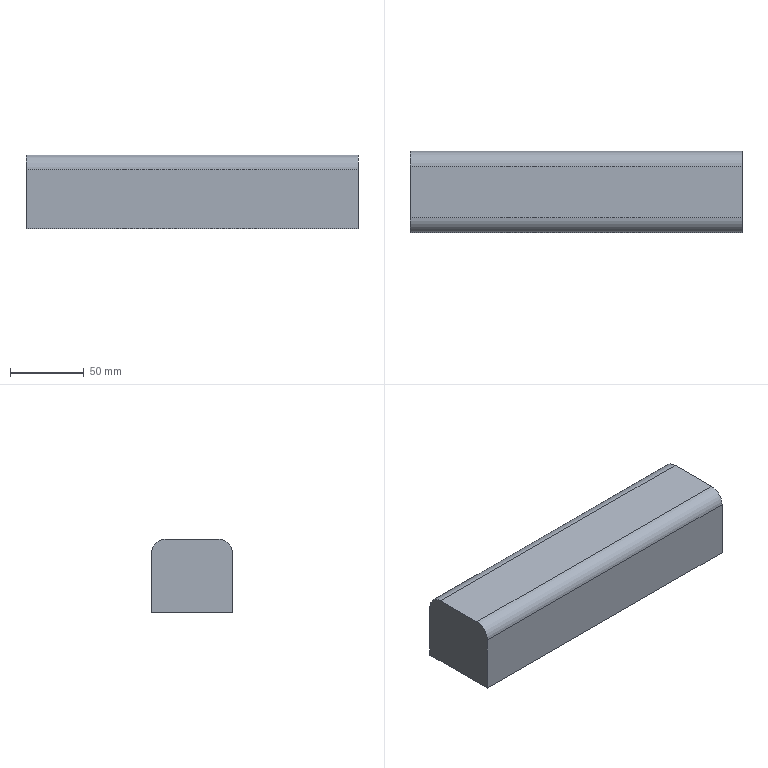Part | NX | features solid 2 | 1 solid | 8 faces | box 225 x 55 x 50 mm | volume 609093 mm3 | plane 6 | cylinder 2 | commonest cylinder face diameters 20 x2
STEP:
#1=CARTESIAN_POINT('',(-55.,-220.,-220.));
#2=VERTEX_POINT('',#1);
#3=CARTESIAN_POINT('',(-55.,-185.,-220.));
#4=VERTEX_POINT('',#3);
#5=CARTESIAN_POINT('',(-55.,-230.,-220.));
#6=DIRECTION('',(0.,-1.,0.));
#7=VECTOR('',#6,1000.);
#8=LINE('',#5,#7);
#9=EDGE_CURVE('',#2,#4,#8,.F.);
#10=ORIENTED_EDGE('',*,*,#9,.T.);
#11=CARTESIAN_POINT('',(-280.,-185.,-220.));
#12=VERTEX_POINT('',#11);
#13=CARTESIAN_POINT('',(-280.,-185.,-220.));
#14=DIRECTION('',(1.,0.,0.));
#15=VECTOR('',#14,1000.);
#16=LINE('',#13,#15);
#17=EDGE_CURVE('',#4,#12,#16,.F.);
#18=ORIENTED_EDGE('',*,*,#17,.T.);
#19=CARTESIAN_POINT('',(-280.,-220.,-220.));
#20=VERTEX_POINT('',#19);
#21=CARTESIAN_POINT('',(-280.,-230.,-220.));
#22=DIRECTION('',(0.,-1.,0.));
#23=VECTOR('',#22,1000.);
#24=LINE('',#21,#23);
#25=EDGE_CURVE('',#20,#12,#24,.F.);
#26=ORIENTED_EDGE('',*,*,#25,.F.);
#27=CARTESIAN_POINT('',(-280.,-220.,-220.));
#28=DIRECTION('',(1.,0.,0.));
#29=VECTOR('',#28,1000.);
#30=LINE('',#27,#29);
#31=EDGE_CURVE('',#20,#2,#30,.T.);
#32=ORIENTED_EDGE('',*,*,#31,.T.);
#33=EDGE_LOOP('',(#10,#18,#26,#32));
#34=FACE_BOUND('',#33,.T.);
#35=CARTESIAN_POINT('',(-280.,-230.,-220.));
#36=DIRECTION('',(0.,0.,1.));
#37=DIRECTION('',(1.,0.,0.));
#38=AXIS2_PLACEMENT_3D('',#35,#36,#37);
#39=PLANE('',#38);
#40=ADVANCED_FACE('',(#34),#39,.T.);
#41=ORIENTED_EDGE('',*,*,#25,.T.);
#42=CARTESIAN_POINT('',(-280.,-175.,-230.));
#43=VERTEX_POINT('',#42);
#44=CARTESIAN_POINT('',(-280.,-185.,-230.));
#45=DIRECTION('',(1.,0.,0.));
#46=DIRECTION('',(0.,0.,-1.));
#47=AXIS2_PLACEMENT_3D('',#44,#45,#46);
#48=CIRCLE('',#47,10.);
#49=EDGE_CURVE('',#12,#43,#48,.F.);
#50=ORIENTED_EDGE('',*,*,#49,.T.);
#51=CARTESIAN_POINT('',(-280.,-175.,-270.));
#52=VERTEX_POINT('',#51);
#53=CARTESIAN_POINT('',(-280.,-175.,-220.));
#54=DIRECTION('',(0.,0.,1.));
#55=VECTOR('',#54,1000.);
#56=LINE('',#53,#55);
#57=EDGE_CURVE('',#43,#52,#56,.F.);
#58=ORIENTED_EDGE('',*,*,#57,.T.);
#59=CARTESIAN_POINT('',(-280.,-230.,-270.));
#60=VERTEX_POINT('',#59);
#61=CARTESIAN_POINT('',(-280.,-230.,-270.));
#62=DIRECTION('',(0.,-1.,0.));
#63=VECTOR('',#62,1000.);
#64=LINE('',#61,#63);
#65=EDGE_CURVE('',#60,#52,#64,.F.);
#66=ORIENTED_EDGE('',*,*,#65,.F.);
#67=CARTESIAN_POINT('',(-280.,-230.,-230.));
#68=VERTEX_POINT('',#67);
#69=CARTESIAN_POINT('',(-280.,-230.,-220.));
#70=DIRECTION('',(0.,0.,-1.));
#71=VECTOR('',#70,1000.);
#72=LINE('',#69,#71);
#73=EDGE_CURVE('',#68,#60,#72,.T.);
#74=ORIENTED_EDGE('',*,*,#73,.F.);
#75=CARTESIAN_POINT('',(-280.,-220.,-230.));
#76=DIRECTION('',(1.,0.,0.));
#77=DIRECTION('',(0.,0.,-1.));
#78=AXIS2_PLACEMENT_3D('',#75,#76,#77);
#79=CIRCLE('',#78,10.);
#80=EDGE_CURVE('',#68,#20,#79,.F.);
#81=ORIENTED_EDGE('',*,*,#80,.T.);
#82=EDGE_LOOP('',(#41,#50,#58,#66,#74,#81));
#83=FACE_BOUND('',#82,.T.);
#84=CARTESIAN_POINT('',(-280.,-230.,-220.));
#85=DIRECTION('',(1.,0.,0.));
#86=DIRECTION('',(0.,0.,-1.));
#87=AXIS2_PLACEMENT_3D('',#84,#85,#86);
#88=PLANE('',#87);
#89=ADVANCED_FACE('',(#83),#88,.F.);
#90=ORIENTED_EDGE('',*,*,#65,.T.);
#91=CARTESIAN_POINT('',(-55.,-175.,-270.));
#92=VERTEX_POINT('',#91);
#93=CARTESIAN_POINT('',(-280.,-175.,-270.));
#94=DIRECTION('',(1.,0.,0.));
#95=VECTOR('',#94,1000.);
#96=LINE('',#93,#95);
#97=EDGE_CURVE('',#52,#92,#96,.T.);
#98=ORIENTED_EDGE('',*,*,#97,.T.);
#99=CARTESIAN_POINT('',(-55.,-230.,-270.));
#100=VERTEX_POINT('',#99);
#101=CARTESIAN_POINT('',(-55.,-230.,-270.));
#102=DIRECTION('',(0.,-1.,0.));
#103=VECTOR('',#102,1000.);
#104=LINE('',#101,#103);
#105=EDGE_CURVE('',#100,#92,#104,.F.);
#106=ORIENTED_EDGE('',*,*,#105,.F.);
#107=CARTESIAN_POINT('',(-280.,-230.,-270.));
#108=DIRECTION('',(1.,0.,0.));
#109=VECTOR('',#108,1000.);
#110=LINE('',#107,#109);
#111=EDGE_CURVE('',#60,#100,#110,.T.);
#112=ORIENTED_EDGE('',*,*,#111,.F.);
#113=EDGE_LOOP('',(#90,#98,#106,#112));
#114=FACE_BOUND('',#113,.T.);
#115=CARTESIAN_POINT('',(-280.,-230.,-270.));
#116=DIRECTION('',(0.,0.,1.));
#117=DIRECTION('',(1.,0.,0.));
#118=AXIS2_PLACEMENT_3D('',#115,#116,#117);
#119=PLANE('',#118);
#120=ADVANCED_FACE('',(#114),#119,.F.);
#121=CARTESIAN_POINT('',(-55.,-175.,-230.));
#122=VERTEX_POINT('',#121);
#123=CARTESIAN_POINT('',(-55.,-175.,-220.));
#124=DIRECTION('',(0.,0.,1.));
#125=VECTOR('',#124,1000.);
#126=LINE('',#123,#125);
#127=EDGE_CURVE('',#122,#92,#126,.F.);
#128=ORIENTED_EDGE('',*,*,#127,.F.);
#129=CARTESIAN_POINT('',(-55.,-185.,-230.));
#130=DIRECTION('',(1.,0.,0.));
#131=DIRECTION('',(0.,0.,-1.));
#132=AXIS2_PLACEMENT_3D('',#129,#130,#131);
#133=CIRCLE('',#132,10.);
#134=EDGE_CURVE('',#122,#4,#133,.T.);
#135=ORIENTED_EDGE('',*,*,#134,.T.);
#136=ORIENTED_EDGE('',*,*,#9,.F.);
#137=CARTESIAN_POINT('',(-55.,-230.,-230.));
#138=VERTEX_POINT('',#137);
#139=CARTESIAN_POINT('',(-55.,-220.,-230.));
#140=DIRECTION('',(1.,0.,0.));
#141=DIRECTION('',(0.,0.,-1.));
#142=AXIS2_PLACEMENT_3D('',#139,#140,#141);
#143=CIRCLE('',#142,10.);
#144=EDGE_CURVE('',#2,#138,#143,.T.);
#145=ORIENTED_EDGE('',*,*,#144,.T.);
#146=CARTESIAN_POINT('',(-55.,-230.,-220.));
#147=DIRECTION('',(0.,0.,-1.));
#148=VECTOR('',#147,1000.);
#149=LINE('',#146,#148);
#150=EDGE_CURVE('',#138,#100,#149,.T.);
#151=ORIENTED_EDGE('',*,*,#150,.T.);
#152=ORIENTED_EDGE('',*,*,#105,.T.);
#153=EDGE_LOOP('',(#128,#135,#136,#145,#151,#152));
#154=FACE_BOUND('',#153,.T.);
#155=CARTESIAN_POINT('',(-55.,-230.,-220.));
#156=DIRECTION('',(1.,0.,0.));
#157=DIRECTION('',(0.,0.,-1.));
#158=AXIS2_PLACEMENT_3D('',#155,#156,#157);
#159=PLANE('',#158);
#160=ADVANCED_FACE('',(#154),#159,.T.);
#161=ORIENTED_EDGE('',*,*,#57,.F.);
#162=CARTESIAN_POINT('',(-55.,-175.,-230.));
#163=DIRECTION('',(-1.,0.,0.));
#164=VECTOR('',#163,1000.);
#165=LINE('',#162,#164);
#166=EDGE_CURVE('',#43,#122,#165,.F.);
#167=ORIENTED_EDGE('',*,*,#166,.T.);
#168=ORIENTED_EDGE('',*,*,#127,.T.);
#169=ORIENTED_EDGE('',*,*,#97,.F.);
#170=EDGE_LOOP('',(#161,#167,#168,#169));
#171=FACE_BOUND('',#170,.T.);
#172=CARTESIAN_POINT('',(-280.,-175.,-220.));
#173=DIRECTION('',(0.,1.,0.));
#174=DIRECTION('',(0.,0.,1.));
#175=AXIS2_PLACEMENT_3D('',#172,#173,#174);
#176=PLANE('',#175);
#177=ADVANCED_FACE('',(#171),#176,.T.);
#178=ORIENTED_EDGE('',*,*,#150,.F.);
#179=CARTESIAN_POINT('',(-280.,-230.,-230.));
#180=DIRECTION('',(-1.,0.,0.));
#181=VECTOR('',#180,1000.);
#182=LINE('',#179,#181);
#183=EDGE_CURVE('',#138,#68,#182,.T.);
#184=ORIENTED_EDGE('',*,*,#183,.T.);
#185=ORIENTED_EDGE('',*,*,#73,.T.);
#186=ORIENTED_EDGE('',*,*,#111,.T.);
#187=EDGE_LOOP('',(#178,#184,#185,#186));
#188=FACE_BOUND('',#187,.T.);
#189=CARTESIAN_POINT('',(-280.,-230.,-220.));
#190=DIRECTION('',(0.,1.,0.));
#191=DIRECTION('',(0.,0.,1.));
#192=AXIS2_PLACEMENT_3D('',#189,#190,#191);
#193=PLANE('',#192);
#194=ADVANCED_FACE('',(#188),#193,.F.);
#195=ORIENTED_EDGE('',*,*,#49,.F.);
#196=ORIENTED_EDGE('',*,*,#17,.F.);
#197=ORIENTED_EDGE('',*,*,#134,.F.);
#198=ORIENTED_EDGE('',*,*,#166,.F.);
#199=EDGE_LOOP('',(#195,#196,#197,#198));
#200=FACE_BOUND('',#199,.T.);
#201=CARTESIAN_POINT('',(-280.,-185.,-230.));
#202=DIRECTION('',(1.,0.,0.));
#203=DIRECTION('',(0.,0.,-1.));
#204=AXIS2_PLACEMENT_3D('',#201,#202,#203);
#205=CYLINDRICAL_SURFACE('',#204,10.);
#206=ADVANCED_FACE('',(#200),#205,.T.);
#207=ORIENTED_EDGE('',*,*,#80,.F.);
#208=ORIENTED_EDGE('',*,*,#183,.F.);
#209=ORIENTED_EDGE('',*,*,#144,.F.);
#210=ORIENTED_EDGE('',*,*,#31,.F.);
#211=EDGE_LOOP('',(#207,#208,#209,#210));
#212=FACE_BOUND('',#211,.T.);
#213=CARTESIAN_POINT('',(-280.,-220.,-230.));
#214=DIRECTION('',(-1.,0.,0.));
#215=DIRECTION('',(0.,0.,1.));
#216=AXIS2_PLACEMENT_3D('',#213,#214,#215);
#217=CYLINDRICAL_SURFACE('',#216,10.);
#218=ADVANCED_FACE('',(#212),#217,.T.);
#219=CLOSED_SHELL('',(#40,#89,#120,#160,#177,#194,#206,#218));
#220=MANIFOLD_SOLID_BREP('',#219);
#221=(LENGTH_UNIT()NAMED_UNIT(*)SI_UNIT(.MILLI.,.METRE.));
#222=UNCERTAINTY_MEASURE_WITH_UNIT(LENGTH_MEASURE(0.00001),#221,'','');
#223=(NAMED_UNIT(*)PLANE_ANGLE_UNIT()SI_UNIT($,.RADIAN.));
#224=(NAMED_UNIT(*)SI_UNIT($,.STERADIAN.)SOLID_ANGLE_UNIT());
#225=(GEOMETRIC_REPRESENTATION_CONTEXT(3)GLOBAL_UNCERTAINTY_ASSIGNED_CONTEXT((#222))GLOBAL_UNIT_ASSIGNED_CONTEXT((#221,#223,#224))REPRESENTATION_CONTEXT('',''));
#226=ADVANCED_BREP_SHAPE_REPRESENTATION('',(#220),#225);